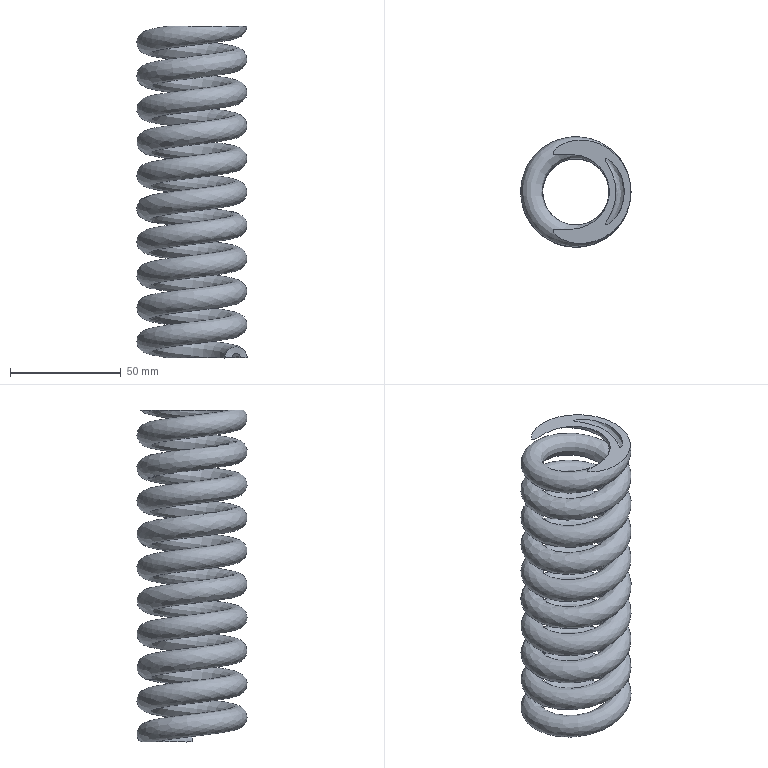Part | NX | features solid 2 | 1 solid | 5 faces | box 49.926 x 49.833 x 150.002 mm | volume 81589 mm3 | spline 3 | plane 2